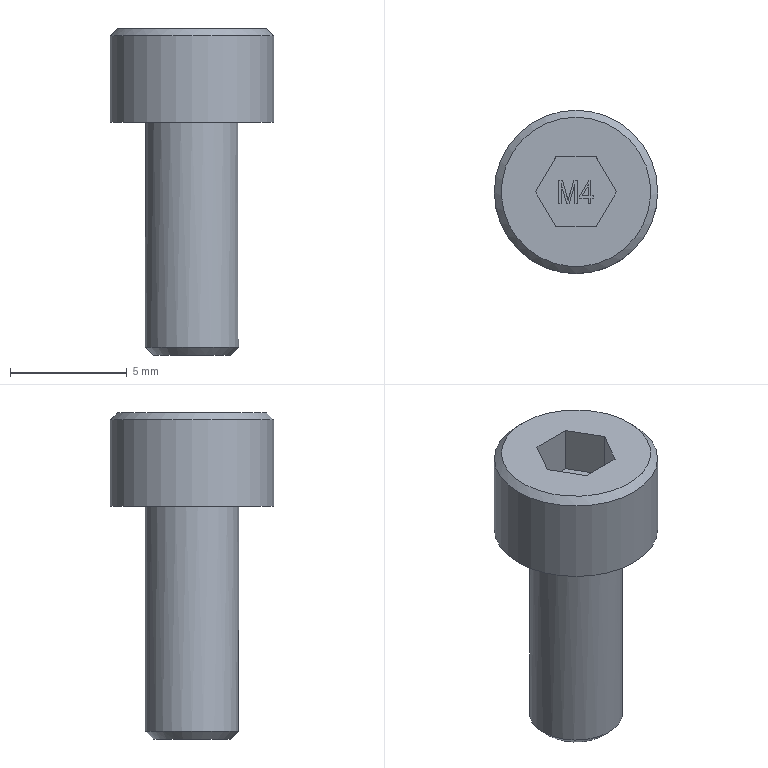Part | STEP file | EM10401000 | 1 solid | 44 faces | box 7 x 7 x 14 mm | volume 262.339 mm3 | plane 38 | cylinder 2 | cone 2 | other 2 | commonest cylinder face diameters 4 x1 7 x1